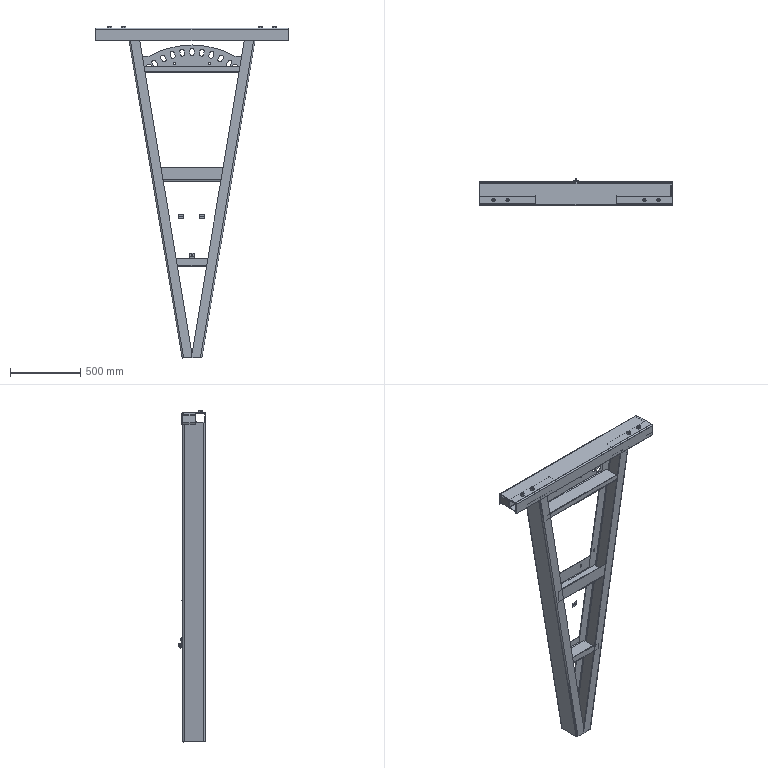Part | SolidWorks | features InContextFeatHolder 8, CompositeCurve 2 | 25 solids | 554 faces | box 1370 x 197 x 2359 mm | volume 12525634 mm3 | plane 284 | cylinder 217 | cone 48 | spline 3 | sphere 2 | commonest cylinder face diameters 6.3 x40 30 x37 20 x31 18 x24 8 x16 10 x16